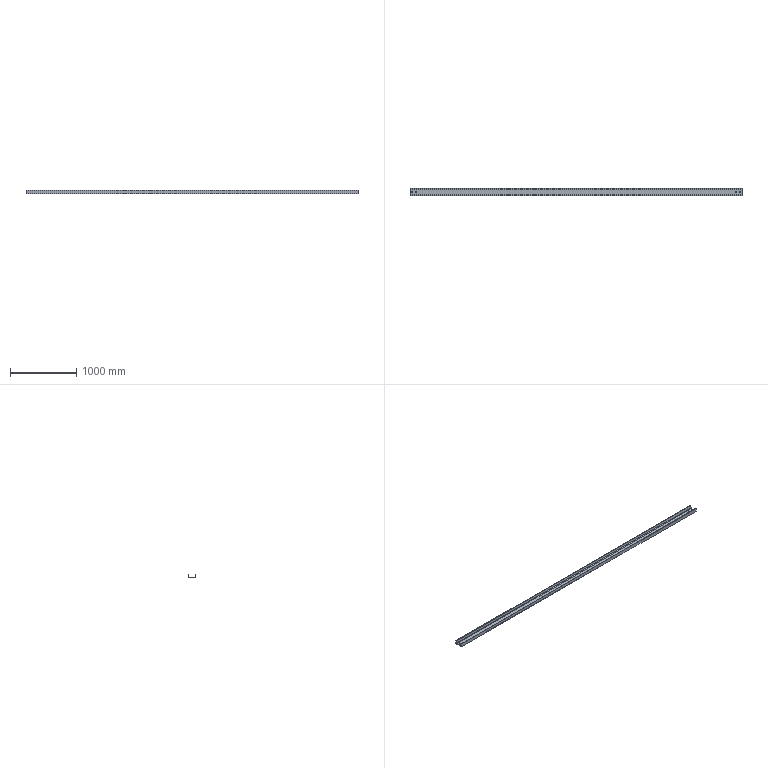Part | STEP file | E3-Transfer kettle connecting beam 2_Default<As Machined> | 1 solid | 22 faces | box 5030 x 120 x 53 mm | volume 7716497 mm3 | cylinder 12 | plane 10 | commonest cylinder face diameters 19 x8 9 x2 18 x2